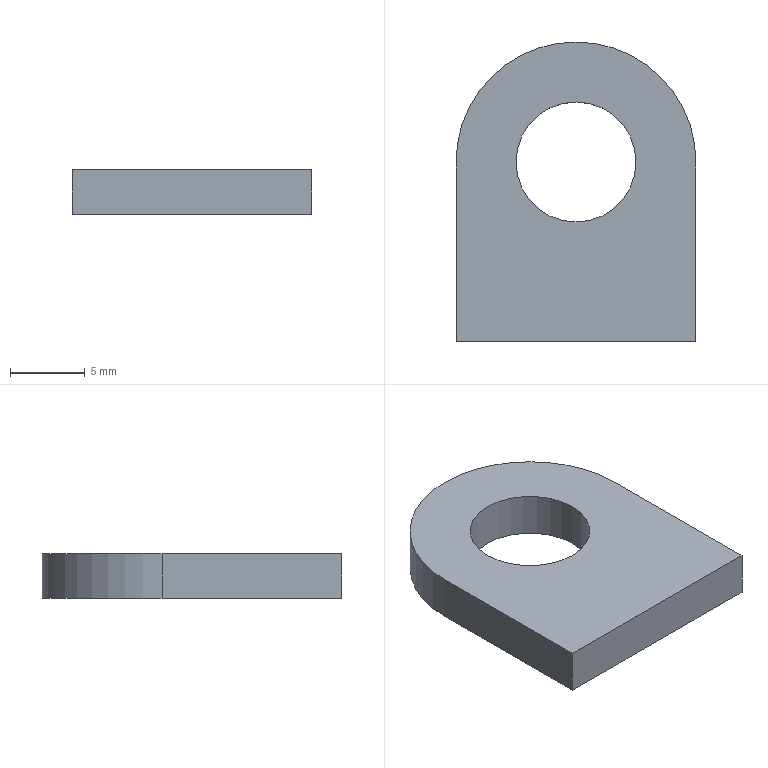Part | NX | features DATUM_CSYS 1, EXTRACT_DATUM_PLANE 1, EXTRUDE 1, SKETCH 1 | 1 solid | 7 faces | box 16 x 20 x 3 mm | volume 726.796 mm3 | plane 5 | cylinder 2 | commonest cylinder face diameters 8 x1 16 x1
STEP:
#1=CARTESIAN_POINT('',(-8.,0.,1.5));
#2=VERTEX_POINT('',#1);
#3=CARTESIAN_POINT('',(-8.,-12.,1.5));
#4=VERTEX_POINT('',#3);
#5=CARTESIAN_POINT('',(-8.,0.,1.5));
#6=DIRECTION('',(0.,-1.,0.));
#7=VECTOR('',#6,1000.);
#8=LINE('',#5,#7);
#9=EDGE_CURVE('',#2,#4,#8,.T.);
#10=ORIENTED_EDGE('',*,*,#9,.F.);
#11=CARTESIAN_POINT('',(-8.,0.,-1.5));
#12=VERTEX_POINT('',#11);
#13=CARTESIAN_POINT('',(-8.,0.,-1.5));
#14=DIRECTION('',(0.,0.,1.));
#15=VECTOR('',#14,1000.);
#16=LINE('',#13,#15);
#17=EDGE_CURVE('',#12,#2,#16,.T.);
#18=ORIENTED_EDGE('',*,*,#17,.F.);
#19=CARTESIAN_POINT('',(-8.,-12.,-1.5));
#20=VERTEX_POINT('',#19);
#21=CARTESIAN_POINT('',(-8.,0.,-1.5));
#22=DIRECTION('',(0.,-1.,0.));
#23=VECTOR('',#22,1000.);
#24=LINE('',#21,#23);
#25=EDGE_CURVE('',#12,#20,#24,.T.);
#26=ORIENTED_EDGE('',*,*,#25,.T.);
#27=CARTESIAN_POINT('',(-8.,-12.,-1.5));
#28=DIRECTION('',(0.,0.,1.));
#29=VECTOR('',#28,1000.);
#30=LINE('',#27,#29);
#31=EDGE_CURVE('',#20,#4,#30,.T.);
#32=ORIENTED_EDGE('',*,*,#31,.T.);
#33=EDGE_LOOP('',(#10,#18,#26,#32));
#34=FACE_BOUND('',#33,.T.);
#35=CARTESIAN_POINT('',(-8.,0.,-1.5));
#36=DIRECTION('',(-1.,0.,0.));
#37=DIRECTION('',(0.,0.,1.));
#38=AXIS2_PLACEMENT_3D('',#35,#36,#37);
#39=PLANE('',#38);
#40=ADVANCED_FACE('',(#34),#39,.T.);
#41=CARTESIAN_POINT('',(8.,-12.,1.5));
#42=VERTEX_POINT('',#41);
#43=CARTESIAN_POINT('',(-8.,-12.,1.5));
#44=DIRECTION('',(1.,0.,0.));
#45=VECTOR('',#44,1000.);
#46=LINE('',#43,#45);
#47=EDGE_CURVE('',#4,#42,#46,.T.);
#48=ORIENTED_EDGE('',*,*,#47,.F.);
#49=ORIENTED_EDGE('',*,*,#31,.F.);
#50=CARTESIAN_POINT('',(8.,-12.,-1.5));
#51=VERTEX_POINT('',#50);
#52=CARTESIAN_POINT('',(-8.,-12.,-1.5));
#53=DIRECTION('',(1.,0.,0.));
#54=VECTOR('',#53,1000.);
#55=LINE('',#52,#54);
#56=EDGE_CURVE('',#20,#51,#55,.T.);
#57=ORIENTED_EDGE('',*,*,#56,.T.);
#58=CARTESIAN_POINT('',(8.,-12.,-1.5));
#59=DIRECTION('',(0.,0.,1.));
#60=VECTOR('',#59,1000.);
#61=LINE('',#58,#60);
#62=EDGE_CURVE('',#51,#42,#61,.T.);
#63=ORIENTED_EDGE('',*,*,#62,.T.);
#64=EDGE_LOOP('',(#48,#49,#57,#63));
#65=FACE_BOUND('',#64,.T.);
#66=CARTESIAN_POINT('',(-8.,-12.,-1.5));
#67=DIRECTION('',(0.,-1.,0.));
#68=DIRECTION('',(0.,0.,-1.));
#69=AXIS2_PLACEMENT_3D('',#66,#67,#68);
#70=PLANE('',#69);
#71=ADVANCED_FACE('',(#65),#70,.T.);
#72=CARTESIAN_POINT('',(8.,0.,1.5));
#73=VERTEX_POINT('',#72);
#74=CARTESIAN_POINT('',(8.,-12.,1.5));
#75=DIRECTION('',(0.,1.,0.));
#76=VECTOR('',#75,1000.);
#77=LINE('',#74,#76);
#78=EDGE_CURVE('',#42,#73,#77,.T.);
#79=ORIENTED_EDGE('',*,*,#78,.F.);
#80=ORIENTED_EDGE('',*,*,#62,.F.);
#81=CARTESIAN_POINT('',(8.,0.,-1.5));
#82=VERTEX_POINT('',#81);
#83=CARTESIAN_POINT('',(8.,-12.,-1.5));
#84=DIRECTION('',(0.,1.,0.));
#85=VECTOR('',#84,1000.);
#86=LINE('',#83,#85);
#87=EDGE_CURVE('',#51,#82,#86,.T.);
#88=ORIENTED_EDGE('',*,*,#87,.T.);
#89=CARTESIAN_POINT('',(8.,0.,-1.5));
#90=DIRECTION('',(0.,0.,1.));
#91=VECTOR('',#90,1000.);
#92=LINE('',#89,#91);
#93=EDGE_CURVE('',#82,#73,#92,.T.);
#94=ORIENTED_EDGE('',*,*,#93,.T.);
#95=EDGE_LOOP('',(#79,#80,#88,#94));
#96=FACE_BOUND('',#95,.T.);
#97=CARTESIAN_POINT('',(8.,-12.,-1.5));
#98=DIRECTION('',(1.,0.,0.));
#99=DIRECTION('',(0.,0.,-1.));
#100=AXIS2_PLACEMENT_3D('',#97,#98,#99);
#101=PLANE('',#100);
#102=ADVANCED_FACE('',(#96),#101,.T.);
#103=CARTESIAN_POINT('',(0.,0.,1.5));
#104=DIRECTION('',(0.,0.,1.));
#105=DIRECTION('',(1.,0.,0.));
#106=AXIS2_PLACEMENT_3D('',#103,#104,#105);
#107=CIRCLE('',#106,8.);
#108=EDGE_CURVE('',#73,#2,#107,.T.);
#109=ORIENTED_EDGE('',*,*,#108,.F.);
#110=ORIENTED_EDGE('',*,*,#93,.F.);
#111=CARTESIAN_POINT('',(0.,0.,-1.5));
#112=DIRECTION('',(0.,0.,1.));
#113=DIRECTION('',(1.,0.,0.));
#114=AXIS2_PLACEMENT_3D('',#111,#112,#113);
#115=CIRCLE('',#114,8.);
#116=EDGE_CURVE('',#82,#12,#115,.T.);
#117=ORIENTED_EDGE('',*,*,#116,.T.);
#118=ORIENTED_EDGE('',*,*,#17,.T.);
#119=EDGE_LOOP('',(#109,#110,#117,#118));
#120=FACE_BOUND('',#119,.T.);
#121=CARTESIAN_POINT('',(0.,0.,-1.5));
#122=DIRECTION('',(0.,0.,1.));
#123=DIRECTION('',(1.,0.,0.));
#124=AXIS2_PLACEMENT_3D('',#121,#122,#123);
#125=CYLINDRICAL_SURFACE('',#124,8.);
#126=ADVANCED_FACE('',(#120),#125,.T.);
#127=CARTESIAN_POINT('',(-4.,0.,1.5));
#128=VERTEX_POINT('',#127);
#129=CARTESIAN_POINT('',(0.,0.,1.5));
#130=DIRECTION('',(0.,0.,-1.));
#131=DIRECTION('',(-1.,0.,0.));
#132=AXIS2_PLACEMENT_3D('',#129,#130,#131);
#133=CIRCLE('',#132,4.);
#134=EDGE_CURVE('',#128,#128,#133,.T.);
#135=ORIENTED_EDGE('',*,*,#134,.F.);
#136=EDGE_LOOP('',(#135));
#137=FACE_BOUND('',#136,.T.);
#138=CARTESIAN_POINT('',(4.,0.,-1.5));
#139=VERTEX_POINT('',#138);
#140=CARTESIAN_POINT('',(0.,0.,-1.5));
#141=DIRECTION('',(0.,0.,-1.));
#142=DIRECTION('',(1.,0.,0.));
#143=AXIS2_PLACEMENT_3D('',#140,#141,#142);
#144=CIRCLE('',#143,4.);
#145=EDGE_CURVE('',#139,#139,#144,.T.);
#146=ORIENTED_EDGE('',*,*,#145,.T.);
#147=EDGE_LOOP('',(#146));
#148=FACE_BOUND('',#147,.T.);
#149=CARTESIAN_POINT('',(0.,0.,-1.5));
#150=DIRECTION('',(0.,0.,1.));
#151=DIRECTION('',(1.,0.,0.));
#152=AXIS2_PLACEMENT_3D('',#149,#150,#151);
#153=CYLINDRICAL_SURFACE('',#152,4.);
#154=ADVANCED_FACE('',(#137,#148),#153,.F.);
#155=ORIENTED_EDGE('',*,*,#25,.F.);
#156=ORIENTED_EDGE('',*,*,#116,.F.);
#157=ORIENTED_EDGE('',*,*,#87,.F.);
#158=ORIENTED_EDGE('',*,*,#56,.F.);
#159=EDGE_LOOP('',(#155,#156,#157,#158));
#160=FACE_BOUND('',#159,.T.);
#161=ORIENTED_EDGE('',*,*,#145,.F.);
#162=EDGE_LOOP('',(#161));
#163=FACE_BOUND('',#162,.T.);
#164=CARTESIAN_POINT('',(0.,0.,-1.5));
#165=DIRECTION('',(0.,0.,1.));
#166=DIRECTION('',(1.,0.,0.));
#167=AXIS2_PLACEMENT_3D('',#164,#165,#166);
#168=PLANE('',#167);
#169=ADVANCED_FACE('',(#160,#163),#168,.F.);
#170=ORIENTED_EDGE('',*,*,#9,.T.);
#171=ORIENTED_EDGE('',*,*,#47,.T.);
#172=ORIENTED_EDGE('',*,*,#78,.T.);
#173=ORIENTED_EDGE('',*,*,#108,.T.);
#174=EDGE_LOOP('',(#170,#171,#172,#173));
#175=FACE_BOUND('',#174,.T.);
#176=ORIENTED_EDGE('',*,*,#134,.T.);
#177=EDGE_LOOP('',(#176));
#178=FACE_BOUND('',#177,.T.);
#179=CARTESIAN_POINT('',(0.,0.,1.5));
#180=DIRECTION('',(0.,0.,1.));
#181=DIRECTION('',(1.,0.,0.));
#182=AXIS2_PLACEMENT_3D('',#179,#180,#181);
#183=PLANE('',#182);
#184=ADVANCED_FACE('',(#175,#178),#183,.T.);
#185=CLOSED_SHELL('',(#40,#71,#102,#126,#154,#169,#184));
#186=MANIFOLD_SOLID_BREP('',#185);
#187=(LENGTH_UNIT()NAMED_UNIT(*)SI_UNIT(.MILLI.,.METRE.));
#188=UNCERTAINTY_MEASURE_WITH_UNIT(LENGTH_MEASURE(0.00001),#187,'','');
#189=(NAMED_UNIT(*)PLANE_ANGLE_UNIT()SI_UNIT($,.RADIAN.));
#190=(NAMED_UNIT(*)SI_UNIT($,.STERADIAN.)SOLID_ANGLE_UNIT());
#191=(GEOMETRIC_REPRESENTATION_CONTEXT(3)GLOBAL_UNCERTAINTY_ASSIGNED_CONTEXT((#188))GLOBAL_UNIT_ASSIGNED_CONTEXT((#187,#189,#190))REPRESENTATION_CONTEXT('',''));
#192=ADVANCED_BREP_SHAPE_REPRESENTATION('',(#186),#191);